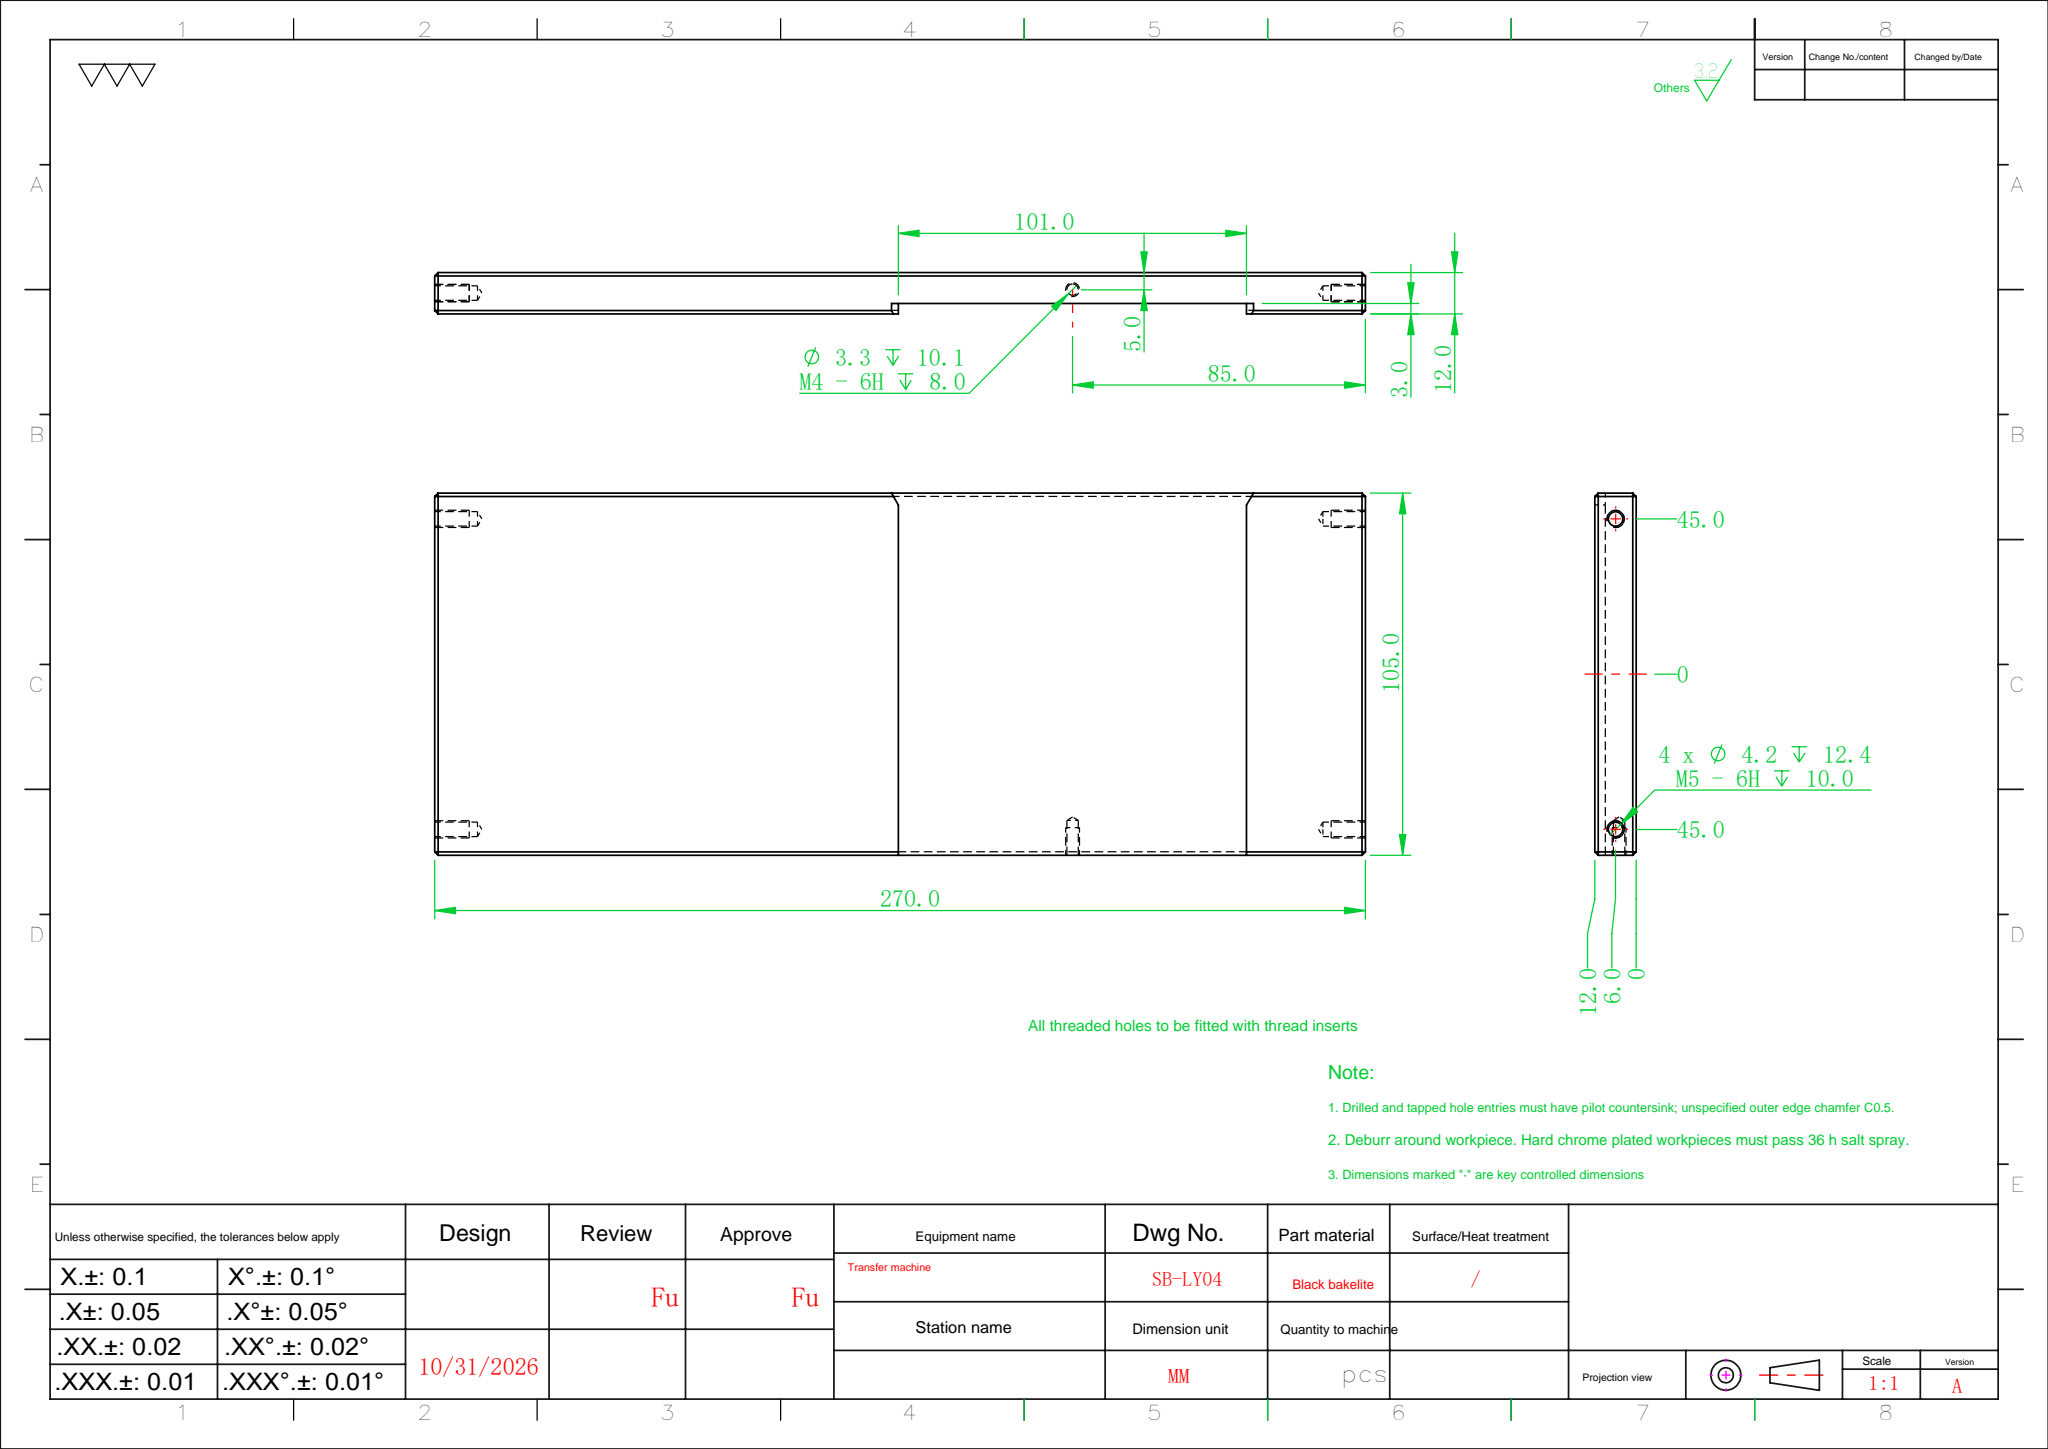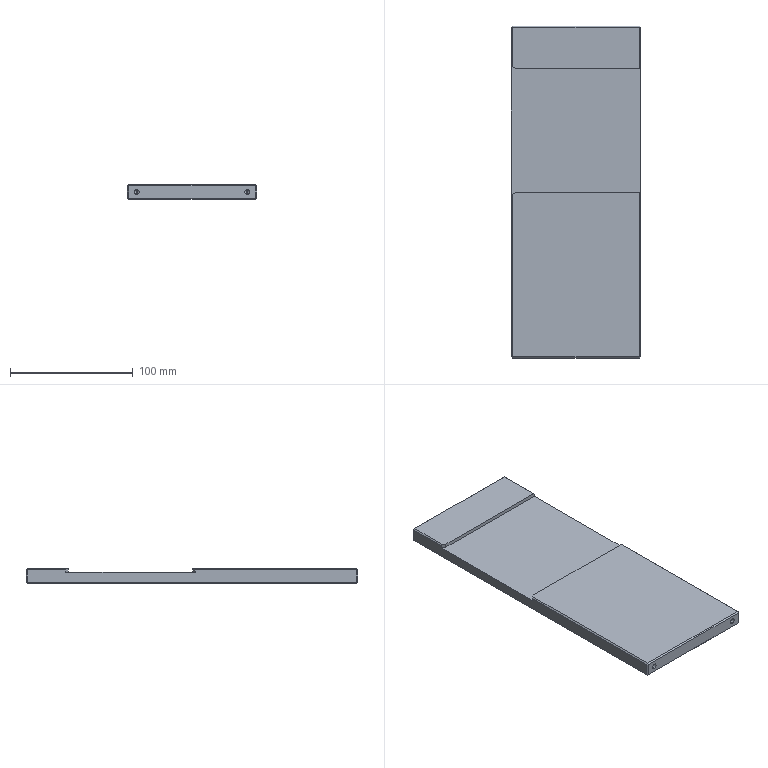Part | SolidWorks | features Chamfer 2, HoleWzd 2, Cut 1, Extrusion 1, MirrorPattern 1 | 1 solid | 54 faces | box 105 x 270 x 12 mm | volume 306899 mm3 | plane 34 | cylinder 10 | cone 10 | commonest cylinder face diameters 4.2 x8 3.3 x2